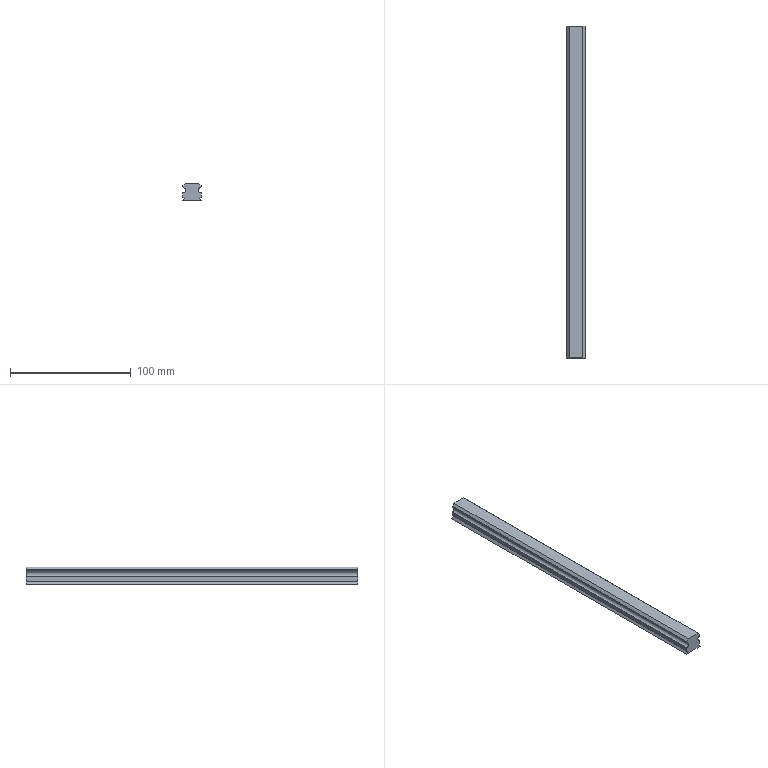Part | NX | features DATUM_CSYS 2, EXTRUDE 1, OFFSET 1, SKETCH 1 | 1 solid | 18 faces | box 16 x 275 x 14.5 mm | volume 53913 mm3 | plane 14 | cylinder 4 | commonest cylinder face diameters 2 x2 4.4 x2
STEP:
#1=CARTESIAN_POINT('',(-6.5,0.,-6.25));
#2=VERTEX_POINT('',#1);
#3=CARTESIAN_POINT('',(-8.,0.,-8.25));
#4=VERTEX_POINT('',#3);
#5=CARTESIAN_POINT('',(-6.5,0.,-6.25));
#6=DIRECTION('',(-0.6,0.,-0.8));
#7=VECTOR('',#6,1000.);
#8=LINE('',#5,#7);
#9=EDGE_CURVE('',#2,#4,#8,.T.);
#10=ORIENTED_EDGE('',*,*,#9,.F.);
#11=CARTESIAN_POINT('',(-6.5,275.,-6.25));
#12=VERTEX_POINT('',#11);
#13=CARTESIAN_POINT('',(-6.5,340.,-6.25));
#14=DIRECTION('',(0.,-1.,0.));
#15=VECTOR('',#14,1000.);
#16=LINE('',#13,#15);
#17=EDGE_CURVE('',#12,#2,#16,.T.);
#18=ORIENTED_EDGE('',*,*,#17,.F.);
#19=CARTESIAN_POINT('',(-8.,275.,-8.25));
#20=VERTEX_POINT('',#19);
#21=CARTESIAN_POINT('',(-6.5,275.,-6.25));
#22=DIRECTION('',(-0.6,0.,-0.8));
#23=VECTOR('',#22,1000.);
#24=LINE('',#21,#23);
#25=EDGE_CURVE('',#12,#20,#24,.T.);
#26=ORIENTED_EDGE('',*,*,#25,.T.);
#27=CARTESIAN_POINT('',(-8.,340.,-8.25));
#28=DIRECTION('',(0.,-1.,0.));
#29=VECTOR('',#28,1000.);
#30=LINE('',#27,#29);
#31=EDGE_CURVE('',#20,#4,#30,.T.);
#32=ORIENTED_EDGE('',*,*,#31,.T.);
#33=EDGE_LOOP('',(#10,#18,#26,#32));
#34=FACE_BOUND('',#33,.T.);
#35=CARTESIAN_POINT('',(-6.5,340.,-6.25));
#36=DIRECTION('',(-0.8,0.,0.6));
#37=DIRECTION('',(0.6,0.,0.8));
#38=AXIS2_PLACEMENT_3D('',#35,#36,#37);
#39=PLANE('',#38);
#40=ADVANCED_FACE('',(#34),#39,.T.);
#41=CARTESIAN_POINT('',(8.,0.,-8.25));
#42=VERTEX_POINT('',#41);
#43=CARTESIAN_POINT('',(0.,0.,-8.25));
#44=DIRECTION('',(1.,0.,0.));
#45=VECTOR('',#44,1000.);
#46=LINE('',#43,#45);
#47=EDGE_CURVE('',#4,#42,#46,.T.);
#48=ORIENTED_EDGE('',*,*,#47,.F.);
#49=ORIENTED_EDGE('',*,*,#31,.F.);
#50=CARTESIAN_POINT('',(8.,275.,-8.25));
#51=VERTEX_POINT('',#50);
#52=CARTESIAN_POINT('',(0.,275.,-8.25));
#53=DIRECTION('',(1.,0.,0.));
#54=VECTOR('',#53,1000.);
#55=LINE('',#52,#54);
#56=EDGE_CURVE('',#20,#51,#55,.T.);
#57=ORIENTED_EDGE('',*,*,#56,.T.);
#58=CARTESIAN_POINT('',(8.,340.,-8.25));
#59=DIRECTION('',(0.,-1.,0.));
#60=VECTOR('',#59,1000.);
#61=LINE('',#58,#60);
#62=EDGE_CURVE('',#51,#42,#61,.T.);
#63=ORIENTED_EDGE('',*,*,#62,.T.);
#64=EDGE_LOOP('',(#48,#49,#57,#63));
#65=FACE_BOUND('',#64,.T.);
#66=CARTESIAN_POINT('',(0.,340.,-8.25));
#67=DIRECTION('',(0.,0.,-1.));
#68=DIRECTION('',(-1.,0.,0.));
#69=AXIS2_PLACEMENT_3D('',#66,#67,#68);
#70=PLANE('',#69);
#71=ADVANCED_FACE('',(#65),#70,.T.);
#72=CARTESIAN_POINT('',(6.5,0.,-6.25));
#73=VERTEX_POINT('',#72);
#74=CARTESIAN_POINT('',(8.,0.,-8.25));
#75=DIRECTION('',(-0.6,0.,0.8));
#76=VECTOR('',#75,1000.);
#77=LINE('',#74,#76);
#78=EDGE_CURVE('',#42,#73,#77,.T.);
#79=ORIENTED_EDGE('',*,*,#78,.F.);
#80=ORIENTED_EDGE('',*,*,#62,.F.);
#81=CARTESIAN_POINT('',(6.5,275.,-6.25));
#82=VERTEX_POINT('',#81);
#83=CARTESIAN_POINT('',(8.,275.,-8.25));
#84=DIRECTION('',(-0.6,0.,0.8));
#85=VECTOR('',#84,1000.);
#86=LINE('',#83,#85);
#87=EDGE_CURVE('',#51,#82,#86,.T.);
#88=ORIENTED_EDGE('',*,*,#87,.T.);
#89=CARTESIAN_POINT('',(6.5,340.,-6.25));
#90=DIRECTION('',(0.,-1.,0.));
#91=VECTOR('',#90,1000.);
#92=LINE('',#89,#91);
#93=EDGE_CURVE('',#82,#73,#92,.T.);
#94=ORIENTED_EDGE('',*,*,#93,.T.);
#95=EDGE_LOOP('',(#79,#80,#88,#94));
#96=FACE_BOUND('',#95,.T.);
#97=CARTESIAN_POINT('',(8.,340.,-8.25));
#98=DIRECTION('',(0.8,0.,0.6));
#99=DIRECTION('',(0.6,0.,-0.8));
#100=AXIS2_PLACEMENT_3D('',#97,#98,#99);
#101=PLANE('',#100);
#102=ADVANCED_FACE('',(#96),#101,.T.);
#103=CARTESIAN_POINT('',(7.5,0.,-5.25));
#104=VERTEX_POINT('',#103);
#105=CARTESIAN_POINT('',(6.5,0.,-6.25));
#106=DIRECTION('',(0.7071,0.,0.7071));
#107=VECTOR('',#106,1000.);
#108=LINE('',#105,#107);
#109=EDGE_CURVE('',#73,#104,#108,.T.);
#110=ORIENTED_EDGE('',*,*,#109,.F.);
#111=ORIENTED_EDGE('',*,*,#93,.F.);
#112=CARTESIAN_POINT('',(7.5,275.,-5.25));
#113=VERTEX_POINT('',#112);
#114=CARTESIAN_POINT('',(6.5,275.,-6.25));
#115=DIRECTION('',(0.7071,0.,0.7071));
#116=VECTOR('',#115,1000.);
#117=LINE('',#114,#116);
#118=EDGE_CURVE('',#82,#113,#117,.T.);
#119=ORIENTED_EDGE('',*,*,#118,.T.);
#120=CARTESIAN_POINT('',(7.5,340.,-5.25));
#121=DIRECTION('',(0.,-1.,0.));
#122=VECTOR('',#121,1000.);
#123=LINE('',#120,#122);
#124=EDGE_CURVE('',#113,#104,#123,.T.);
#125=ORIENTED_EDGE('',*,*,#124,.T.);
#126=EDGE_LOOP('',(#110,#111,#119,#125));
#127=FACE_BOUND('',#126,.T.);
#128=CARTESIAN_POINT('',(6.5,340.,-6.25));
#129=DIRECTION('',(0.7071,0.,-0.7071));
#130=DIRECTION('',(-0.7071,0.,-0.7071));
#131=AXIS2_PLACEMENT_3D('',#128,#129,#130);
#132=PLANE('',#131);
#133=ADVANCED_FACE('',(#127),#132,.T.);
#134=CARTESIAN_POINT('',(7.5,0.,-1.75));
#135=VERTEX_POINT('',#134);
#136=CARTESIAN_POINT('',(7.5,0.,-5.25));
#137=DIRECTION('',(0.,0.,1.));
#138=VECTOR('',#137,1000.);
#139=LINE('',#136,#138);
#140=EDGE_CURVE('',#104,#135,#139,.T.);
#141=ORIENTED_EDGE('',*,*,#140,.F.);
#142=ORIENTED_EDGE('',*,*,#124,.F.);
#143=CARTESIAN_POINT('',(7.5,275.,-1.75));
#144=VERTEX_POINT('',#143);
#145=CARTESIAN_POINT('',(7.5,275.,-5.25));
#146=DIRECTION('',(0.,0.,1.));
#147=VECTOR('',#146,1000.);
#148=LINE('',#145,#147);
#149=EDGE_CURVE('',#113,#144,#148,.T.);
#150=ORIENTED_EDGE('',*,*,#149,.T.);
#151=CARTESIAN_POINT('',(7.5,340.,-1.75));
#152=DIRECTION('',(0.,-1.,0.));
#153=VECTOR('',#152,1000.);
#154=LINE('',#151,#153);
#155=EDGE_CURVE('',#144,#135,#154,.T.);
#156=ORIENTED_EDGE('',*,*,#155,.T.);
#157=EDGE_LOOP('',(#141,#142,#150,#156));
#158=FACE_BOUND('',#157,.T.);
#159=CARTESIAN_POINT('',(7.5,340.,-5.25));
#160=DIRECTION('',(1.,0.,0.));
#161=DIRECTION('',(0.,0.,-1.));
#162=AXIS2_PLACEMENT_3D('',#159,#160,#161);
#163=PLANE('',#162);
#164=ADVANCED_FACE('',(#158),#163,.T.);
#165=CARTESIAN_POINT('',(6.813,0.,2.54));
#166=VERTEX_POINT('',#165);
#167=CARTESIAN_POINT('',(7.5,0.,0.45));
#168=DIRECTION('',(0.,1.,0.));
#169=DIRECTION('',(1.,0.,0.));
#170=AXIS2_PLACEMENT_3D('',#167,#168,#169);
#171=CIRCLE('',#170,2.2);
#172=EDGE_CURVE('',#135,#166,#171,.T.);
#173=ORIENTED_EDGE('',*,*,#172,.F.);
#174=ORIENTED_EDGE('',*,*,#155,.F.);
#175=CARTESIAN_POINT('',(6.813,275.,2.54));
#176=VERTEX_POINT('',#175);
#177=CARTESIAN_POINT('',(7.5,275.,0.45));
#178=DIRECTION('',(0.,1.,0.));
#179=DIRECTION('',(0.,0.,1.));
#180=AXIS2_PLACEMENT_3D('',#177,#178,#179);
#181=CIRCLE('',#180,2.2);
#182=EDGE_CURVE('',#144,#176,#181,.T.);
#183=ORIENTED_EDGE('',*,*,#182,.T.);
#184=CARTESIAN_POINT('',(6.813,340.,2.54));
#185=DIRECTION('',(0.,-1.,0.));
#186=VECTOR('',#185,1000.);
#187=LINE('',#184,#186);
#188=EDGE_CURVE('',#176,#166,#187,.T.);
#189=ORIENTED_EDGE('',*,*,#188,.T.);
#190=EDGE_LOOP('',(#173,#174,#183,#189));
#191=FACE_BOUND('',#190,.T.);
#192=CARTESIAN_POINT('',(7.5,340.,0.45));
#193=DIRECTION('',(0.,-1.,0.));
#194=DIRECTION('',(0.,0.,-1.));
#195=AXIS2_PLACEMENT_3D('',#192,#193,#194);
#196=CYLINDRICAL_SURFACE('',#195,2.2);
#197=ADVANCED_FACE('',(#191),#196,.F.);
#198=CARTESIAN_POINT('',(7.5,0.,3.49));
#199=VERTEX_POINT('',#198);
#200=CARTESIAN_POINT('',(6.5,0.,3.49));
#201=DIRECTION('',(0.,-1.,0.));
#202=DIRECTION('',(1.,0.,0.));
#203=AXIS2_PLACEMENT_3D('',#200,#201,#202);
#204=CIRCLE('',#203,1.);
#205=EDGE_CURVE('',#166,#199,#204,.T.);
#206=ORIENTED_EDGE('',*,*,#205,.F.);
#207=ORIENTED_EDGE('',*,*,#188,.F.);
#208=CARTESIAN_POINT('',(7.5,275.,3.49));
#209=VERTEX_POINT('',#208);
#210=CARTESIAN_POINT('',(6.5,275.,3.49));
#211=DIRECTION('',(0.,1.,0.));
#212=DIRECTION('',(0.,0.,1.));
#213=AXIS2_PLACEMENT_3D('',#210,#211,#212);
#214=CIRCLE('',#213,1.);
#215=EDGE_CURVE('',#176,#209,#214,.F.);
#216=ORIENTED_EDGE('',*,*,#215,.T.);
#217=CARTESIAN_POINT('',(7.5,340.,3.49));
#218=DIRECTION('',(0.,-1.,0.));
#219=VECTOR('',#218,1000.);
#220=LINE('',#217,#219);
#221=EDGE_CURVE('',#209,#199,#220,.T.);
#222=ORIENTED_EDGE('',*,*,#221,.T.);
#223=EDGE_LOOP('',(#206,#207,#216,#222));
#224=FACE_BOUND('',#223,.T.);
#225=CARTESIAN_POINT('',(6.5,340.,3.49));
#226=DIRECTION('',(0.,-1.,0.));
#227=DIRECTION('',(0.,0.,-1.));
#228=AXIS2_PLACEMENT_3D('',#225,#226,#227);
#229=CYLINDRICAL_SURFACE('',#228,1.);
#230=ADVANCED_FACE('',(#224),#229,.T.);
#231=CARTESIAN_POINT('',(7.5,0.,4.25));
#232=VERTEX_POINT('',#231);
#233=CARTESIAN_POINT('',(7.5,0.,3.49));
#234=DIRECTION('',(0.,0.,1.));
#235=VECTOR('',#234,1000.);
#236=LINE('',#233,#235);
#237=EDGE_CURVE('',#199,#232,#236,.T.);
#238=ORIENTED_EDGE('',*,*,#237,.F.);
#239=ORIENTED_EDGE('',*,*,#221,.F.);
#240=CARTESIAN_POINT('',(7.5,275.,4.25));
#241=VERTEX_POINT('',#240);
#242=CARTESIAN_POINT('',(7.5,275.,3.49));
#243=DIRECTION('',(0.,0.,1.));
#244=VECTOR('',#243,1000.);
#245=LINE('',#242,#244);
#246=EDGE_CURVE('',#209,#241,#245,.T.);
#247=ORIENTED_EDGE('',*,*,#246,.T.);
#248=CARTESIAN_POINT('',(7.5,340.,4.25));
#249=DIRECTION('',(0.,-1.,0.));
#250=VECTOR('',#249,1000.);
#251=LINE('',#248,#250);
#252=EDGE_CURVE('',#241,#232,#251,.T.);
#253=ORIENTED_EDGE('',*,*,#252,.T.);
#254=EDGE_LOOP('',(#238,#239,#247,#253));
#255=FACE_BOUND('',#254,.T.);
#256=CARTESIAN_POINT('',(7.5,340.,3.49));
#257=DIRECTION('',(1.,0.,0.));
#258=DIRECTION('',(0.,0.,-1.));
#259=AXIS2_PLACEMENT_3D('',#256,#257,#258);
#260=PLANE('',#259);
#261=ADVANCED_FACE('',(#255),#260,.T.);
#262=CARTESIAN_POINT('',(5.5,0.,6.25));
#263=VERTEX_POINT('',#262);
#264=CARTESIAN_POINT('',(7.5,0.,4.25));
#265=DIRECTION('',(-0.7071,0.,0.7071));
#266=VECTOR('',#265,1000.);
#267=LINE('',#264,#266);
#268=EDGE_CURVE('',#232,#263,#267,.T.);
#269=ORIENTED_EDGE('',*,*,#268,.F.);
#270=ORIENTED_EDGE('',*,*,#252,.F.);
#271=CARTESIAN_POINT('',(5.5,275.,6.25));
#272=VERTEX_POINT('',#271);
#273=CARTESIAN_POINT('',(7.5,275.,4.25));
#274=DIRECTION('',(-0.7071,0.,0.7071));
#275=VECTOR('',#274,1000.);
#276=LINE('',#273,#275);
#277=EDGE_CURVE('',#241,#272,#276,.T.);
#278=ORIENTED_EDGE('',*,*,#277,.T.);
#279=CARTESIAN_POINT('',(5.5,340.,6.25));
#280=DIRECTION('',(0.,-1.,0.));
#281=VECTOR('',#280,1000.);
#282=LINE('',#279,#281);
#283=EDGE_CURVE('',#272,#263,#282,.T.);
#284=ORIENTED_EDGE('',*,*,#283,.T.);
#285=EDGE_LOOP('',(#269,#270,#278,#284));
#286=FACE_BOUND('',#285,.T.);
#287=CARTESIAN_POINT('',(7.5,340.,4.25));
#288=DIRECTION('',(0.7071,0.,0.7071));
#289=DIRECTION('',(0.7071,0.,-0.7071));
#290=AXIS2_PLACEMENT_3D('',#287,#288,#289);
#291=PLANE('',#290);
#292=ADVANCED_FACE('',(#286),#291,.T.);
#293=CARTESIAN_POINT('',(-5.5,0.,6.25));
#294=VERTEX_POINT('',#293);
#295=CARTESIAN_POINT('',(5.5,0.,6.25));
#296=DIRECTION('',(-1.,0.,0.));
#297=VECTOR('',#296,1000.);
#298=LINE('',#295,#297);
#299=EDGE_CURVE('',#263,#294,#298,.T.);
#300=ORIENTED_EDGE('',*,*,#299,.F.);
#301=ORIENTED_EDGE('',*,*,#283,.F.);
#302=CARTESIAN_POINT('',(-5.5,275.,6.25));
#303=VERTEX_POINT('',#302);
#304=CARTESIAN_POINT('',(5.5,275.,6.25));
#305=DIRECTION('',(-1.,0.,0.));
#306=VECTOR('',#305,1000.);
#307=LINE('',#304,#306);
#308=EDGE_CURVE('',#272,#303,#307,.T.);
#309=ORIENTED_EDGE('',*,*,#308,.T.);
#310=CARTESIAN_POINT('',(-5.5,340.,6.25));
#311=DIRECTION('',(0.,-1.,0.));
#312=VECTOR('',#311,1000.);
#313=LINE('',#310,#312);
#314=EDGE_CURVE('',#303,#294,#313,.T.);
#315=ORIENTED_EDGE('',*,*,#314,.T.);
#316=EDGE_LOOP('',(#300,#301,#309,#315));
#317=FACE_BOUND('',#316,.T.);
#318=CARTESIAN_POINT('',(5.5,340.,6.25));
#319=DIRECTION('',(0.,0.,1.));
#320=DIRECTION('',(1.,0.,0.));
#321=AXIS2_PLACEMENT_3D('',#318,#319,#320);
#322=PLANE('',#321);
#323=ADVANCED_FACE('',(#317),#322,.T.);
#324=CARTESIAN_POINT('',(-7.5,0.,4.25));
#325=VERTEX_POINT('',#324);
#326=CARTESIAN_POINT('',(-5.5,0.,6.25));
#327=DIRECTION('',(-0.7071,0.,-0.7071));
#328=VECTOR('',#327,1000.);
#329=LINE('',#326,#328);
#330=EDGE_CURVE('',#294,#325,#329,.T.);
#331=ORIENTED_EDGE('',*,*,#330,.F.);
#332=ORIENTED_EDGE('',*,*,#314,.F.);
#333=CARTESIAN_POINT('',(-7.5,275.,4.25));
#334=VERTEX_POINT('',#333);
#335=CARTESIAN_POINT('',(-5.5,275.,6.25));
#336=DIRECTION('',(-0.7071,0.,-0.7071));
#337=VECTOR('',#336,1000.);
#338=LINE('',#335,#337);
#339=EDGE_CURVE('',#303,#334,#338,.T.);
#340=ORIENTED_EDGE('',*,*,#339,.T.);
#341=CARTESIAN_POINT('',(-7.5,340.,4.25));
#342=DIRECTION('',(0.,-1.,0.));
#343=VECTOR('',#342,1000.);
#344=LINE('',#341,#343);
#345=EDGE_CURVE('',#334,#325,#344,.T.);
#346=ORIENTED_EDGE('',*,*,#345,.T.);
#347=EDGE_LOOP('',(#331,#332,#340,#346));
#348=FACE_BOUND('',#347,.T.);
#349=CARTESIAN_POINT('',(-5.5,340.,6.25));
#350=DIRECTION('',(-0.7071,0.,0.7071));
#351=DIRECTION('',(0.7071,0.,0.7071));
#352=AXIS2_PLACEMENT_3D('',#349,#350,#351);
#353=PLANE('',#352);
#354=ADVANCED_FACE('',(#348),#353,.T.);
#355=CARTESIAN_POINT('',(-7.5,0.,3.469));
#356=VERTEX_POINT('',#355);
#357=CARTESIAN_POINT('',(-7.5,0.,4.25));
#358=DIRECTION('',(0.,0.,-1.));
#359=VECTOR('',#358,1000.);
#360=LINE('',#357,#359);
#361=EDGE_CURVE('',#325,#356,#360,.T.);
#362=ORIENTED_EDGE('',*,*,#361,.F.);
#363=ORIENTED_EDGE('',*,*,#345,.F.);
#364=CARTESIAN_POINT('',(-7.5,275.,3.469));
#365=VERTEX_POINT('',#364);
#366=CARTESIAN_POINT('',(-7.5,275.,4.25));
#367=DIRECTION('',(0.,0.,-1.));
#368=VECTOR('',#367,1000.);
#369=LINE('',#366,#368);
#370=EDGE_CURVE('',#334,#365,#369,.T.);
#371=ORIENTED_EDGE('',*,*,#370,.T.);
#372=CARTESIAN_POINT('',(-7.5,340.,3.469));
#373=DIRECTION('',(0.,-1.,0.));
#374=VECTOR('',#373,1000.);
#375=LINE('',#372,#374);
#376=EDGE_CURVE('',#365,#356,#375,.T.);
#377=ORIENTED_EDGE('',*,*,#376,.T.);
#378=EDGE_LOOP('',(#362,#363,#371,#377));
#379=FACE_BOUND('',#378,.T.);
#380=CARTESIAN_POINT('',(-7.5,340.,4.25));
#381=DIRECTION('',(-1.,0.,0.));
#382=DIRECTION('',(0.,0.,1.));
#383=AXIS2_PLACEMENT_3D('',#380,#381,#382);
#384=PLANE('',#383);
#385=ADVANCED_FACE('',(#379),#384,.T.);
#386=CARTESIAN_POINT('',(-6.812,0.,2.519));
#387=VERTEX_POINT('',#386);
#388=CARTESIAN_POINT('',(-6.5,0.,3.469));
#389=DIRECTION('',(0.,-1.,0.));
#390=DIRECTION('',(1.,0.,0.));
#391=AXIS2_PLACEMENT_3D('',#388,#389,#390);
#392=CIRCLE('',#391,1.);
#393=EDGE_CURVE('',#356,#387,#392,.T.);
#394=ORIENTED_EDGE('',*,*,#393,.F.);
#395=ORIENTED_EDGE('',*,*,#376,.F.);
#396=CARTESIAN_POINT('',(-6.812,275.,2.519));
#397=VERTEX_POINT('',#396);
#398=CARTESIAN_POINT('',(-6.5,275.,3.469));
#399=DIRECTION('',(0.,1.,0.));
#400=DIRECTION('',(0.,0.,1.));
#401=AXIS2_PLACEMENT_3D('',#398,#399,#400);
#402=CIRCLE('',#401,1.);
#403=EDGE_CURVE('',#365,#397,#402,.F.);
#404=ORIENTED_EDGE('',*,*,#403,.T.);
#405=CARTESIAN_POINT('',(-6.812,340.,2.519));
#406=DIRECTION('',(0.,-1.,0.));
#407=VECTOR('',#406,1000.);
#408=LINE('',#405,#407);
#409=EDGE_CURVE('',#397,#387,#408,.T.);
#410=ORIENTED_EDGE('',*,*,#409,.T.);
#411=EDGE_LOOP('',(#394,#395,#404,#410));
#412=FACE_BOUND('',#411,.T.);
#413=CARTESIAN_POINT('',(-6.5,340.,3.469));
#414=DIRECTION('',(0.,-1.,0.));
#415=DIRECTION('',(0.,0.,-1.));
#416=AXIS2_PLACEMENT_3D('',#413,#414,#415);
#417=CYLINDRICAL_SURFACE('',#416,1.);
#418=ADVANCED_FACE('',(#412),#417,.T.);
#419=CARTESIAN_POINT('',(-7.5,0.,-1.771));
#420=VERTEX_POINT('',#419);
#421=CARTESIAN_POINT('',(-7.5,0.,0.4293));
#422=DIRECTION('',(0.,1.,0.));
#423=DIRECTION('',(1.,0.,0.));
#424=AXIS2_PLACEMENT_3D('',#421,#422,#423);
#425=CIRCLE('',#424,2.2);
#426=EDGE_CURVE('',#387,#420,#425,.T.);
#427=ORIENTED_EDGE('',*,*,#426,.F.);
#428=ORIENTED_EDGE('',*,*,#409,.F.);
#429=CARTESIAN_POINT('',(-7.5,275.,-1.771));
#430=VERTEX_POINT('',#429);
#431=CARTESIAN_POINT('',(-7.5,275.,0.4293));
#432=DIRECTION('',(0.,1.,0.));
#433=DIRECTION('',(0.,0.,1.));
#434=AXIS2_PLACEMENT_3D('',#431,#432,#433);
#435=CIRCLE('',#434,2.2);
#436=EDGE_CURVE('',#397,#430,#435,.T.);
#437=ORIENTED_EDGE('',*,*,#436,.T.);
#438=CARTESIAN_POINT('',(-7.5,340.,-1.771));
#439=DIRECTION('',(0.,-1.,0.));
#440=VECTOR('',#439,1000.);
#441=LINE('',#438,#440);
#442=EDGE_CURVE('',#430,#420,#441,.T.);
#443=ORIENTED_EDGE('',*,*,#442,.T.);
#444=EDGE_LOOP('',(#427,#428,#437,#443));
#445=FACE_BOUND('',#444,.T.);
#446=CARTESIAN_POINT('',(-7.5,340.,0.4293));
#447=DIRECTION('',(0.,-1.,0.));
#448=DIRECTION('',(0.,0.,-1.));
#449=AXIS2_PLACEMENT_3D('',#446,#447,#448);
#450=CYLINDRICAL_SURFACE('',#449,2.2);
#451=ADVANCED_FACE('',(#445),#450,.F.);
#452=CARTESIAN_POINT('',(-7.5,0.,-5.25));
#453=VERTEX_POINT('',#452);
#454=CARTESIAN_POINT('',(-7.5,0.,-1.771));
#455=DIRECTION('',(0.,0.,-1.));
#456=VECTOR('',#455,1000.);
#457=LINE('',#454,#456);
#458=EDGE_CURVE('',#420,#453,#457,.T.);
#459=ORIENTED_EDGE('',*,*,#458,.F.);
#460=ORIENTED_EDGE('',*,*,#442,.F.);
#461=CARTESIAN_POINT('',(-7.5,275.,-5.25));
#462=VERTEX_POINT('',#461);
#463=CARTESIAN_POINT('',(-7.5,275.,-1.771));
#464=DIRECTION('',(0.,0.,-1.));
#465=VECTOR('',#464,1000.);
#466=LINE('',#463,#465);
#467=EDGE_CURVE('',#430,#462,#466,.T.);
#468=ORIENTED_EDGE('',*,*,#467,.T.);
#469=CARTESIAN_POINT('',(-7.5,340.,-5.25));
#470=DIRECTION('',(0.,-1.,0.));
#471=VECTOR('',#470,1000.);
#472=LINE('',#469,#471);
#473=EDGE_CURVE('',#462,#453,#472,.T.);
#474=ORIENTED_EDGE('',*,*,#473,.T.);
#475=EDGE_LOOP('',(#459,#460,#468,#474));
#476=FACE_BOUND('',#475,.T.);
#477=CARTESIAN_POINT('',(-7.5,340.,-1.771));
#478=DIRECTION('',(-1.,0.,0.));
#479=DIRECTION('',(0.,0.,1.));
#480=AXIS2_PLACEMENT_3D('',#477,#478,#479);
#481=PLANE('',#480);
#482=ADVANCED_FACE('',(#476),#481,.T.);
#483=CARTESIAN_POINT('',(-7.5,0.,-5.25));
#484=DIRECTION('',(0.7071,0.,-0.7071));
#485=VECTOR('',#484,1000.);
#486=LINE('',#483,#485);
#487=EDGE_CURVE('',#453,#2,#486,.T.);
#488=ORIENTED_EDGE('',*,*,#487,.F.);
#489=ORIENTED_EDGE('',*,*,#473,.F.);
#490=CARTESIAN_POINT('',(-7.5,275.,-5.25));
#491=DIRECTION('',(0.7071,0.,-0.7071));
#492=VECTOR('',#491,1000.);
#493=LINE('',#490,#492);
#494=EDGE_CURVE('',#462,#12,#493,.T.);
#495=ORIENTED_EDGE('',*,*,#494,.T.);
#496=ORIENTED_EDGE('',*,*,#17,.T.);
#497=EDGE_LOOP('',(#488,#489,#495,#496));
#498=FACE_BOUND('',#497,.T.);
#499=CARTESIAN_POINT('',(-7.5,340.,-5.25));
#500=DIRECTION('',(-0.7071,0.,-0.7071));
#501=DIRECTION('',(-0.7071,0.,0.7071));
#502=AXIS2_PLACEMENT_3D('',#499,#500,#501);
#503=PLANE('',#502);
#504=ADVANCED_FACE('',(#498),#503,.T.);
#505=ORIENTED_EDGE('',*,*,#25,.F.);
#506=ORIENTED_EDGE('',*,*,#494,.F.);
#507=ORIENTED_EDGE('',*,*,#467,.F.);
#508=ORIENTED_EDGE('',*,*,#436,.F.);
#509=ORIENTED_EDGE('',*,*,#403,.F.);
#510=ORIENTED_EDGE('',*,*,#370,.F.);
#511=ORIENTED_EDGE('',*,*,#339,.F.);
#512=ORIENTED_EDGE('',*,*,#308,.F.);
#513=ORIENTED_EDGE('',*,*,#277,.F.);
#514=ORIENTED_EDGE('',*,*,#246,.F.);
#515=ORIENTED_EDGE('',*,*,#215,.F.);
#516=ORIENTED_EDGE('',*,*,#182,.F.);
#517=ORIENTED_EDGE('',*,*,#149,.F.);
#518=ORIENTED_EDGE('',*,*,#118,.F.);
#519=ORIENTED_EDGE('',*,*,#87,.F.);
#520=ORIENTED_EDGE('',*,*,#56,.F.);
#521=EDGE_LOOP('',(#505,#506,#507,#508,#509,#510,#511,#512,#513,#514,#515,#516,#517,#518,#519,#520));
#522=FACE_BOUND('',#521,.T.);
#523=CARTESIAN_POINT('',(7.5,275.,0.45));
#524=DIRECTION('',(0.,1.,0.));
#525=DIRECTION('',(0.,0.,1.));
#526=AXIS2_PLACEMENT_3D('',#523,#524,#525);
#527=PLANE('',#526);
#528=ADVANCED_FACE('',(#522),#527,.T.);
#529=ORIENTED_EDGE('',*,*,#9,.T.);
#530=ORIENTED_EDGE('',*,*,#47,.T.);
#531=ORIENTED_EDGE('',*,*,#78,.T.);
#532=ORIENTED_EDGE('',*,*,#109,.T.);
#533=ORIENTED_EDGE('',*,*,#140,.T.);
#534=ORIENTED_EDGE('',*,*,#172,.T.);
#535=ORIENTED_EDGE('',*,*,#205,.T.);
#536=ORIENTED_EDGE('',*,*,#237,.T.);
#537=ORIENTED_EDGE('',*,*,#268,.T.);
#538=ORIENTED_EDGE('',*,*,#299,.T.);
#539=ORIENTED_EDGE('',*,*,#330,.T.);
#540=ORIENTED_EDGE('',*,*,#361,.T.);
#541=ORIENTED_EDGE('',*,*,#393,.T.);
#542=ORIENTED_EDGE('',*,*,#426,.T.);
#543=ORIENTED_EDGE('',*,*,#458,.T.);
#544=ORIENTED_EDGE('',*,*,#487,.T.);
#545=EDGE_LOOP('',(#529,#530,#531,#532,#533,#534,#535,#536,#537,#538,#539,#540,#541,#542,#543,#544));
#546=FACE_BOUND('',#545,.T.);
#547=CARTESIAN_POINT('',(7.5,0.,0.45));
#548=DIRECTION('',(0.,1.,0.));
#549=DIRECTION('',(0.,0.,1.));
#550=AXIS2_PLACEMENT_3D('',#547,#548,#549);
#551=PLANE('',#550);
#552=ADVANCED_FACE('',(#546),#551,.F.);
#553=CLOSED_SHELL('',(#40,#71,#102,#133,#164,#197,#230,#261,#292,#323,#354,#385,#418,#451,#482,#504,#528,#552));
#554=MANIFOLD_SOLID_BREP('',#553);
#555=(LENGTH_UNIT()NAMED_UNIT(*)SI_UNIT(.MILLI.,.METRE.));
#556=UNCERTAINTY_MEASURE_WITH_UNIT(LENGTH_MEASURE(0.00001),#555,'','');
#557=(NAMED_UNIT(*)PLANE_ANGLE_UNIT()SI_UNIT($,.RADIAN.));
#558=(NAMED_UNIT(*)SI_UNIT($,.STERADIAN.)SOLID_ANGLE_UNIT());
#559=(GEOMETRIC_REPRESENTATION_CONTEXT(3)GLOBAL_UNCERTAINTY_ASSIGNED_CONTEXT((#556))GLOBAL_UNIT_ASSIGNED_CONTEXT((#555,#557,#558))REPRESENTATION_CONTEXT('',''));
#560=ADVANCED_BREP_SHAPE_REPRESENTATION('',(#554),#559);